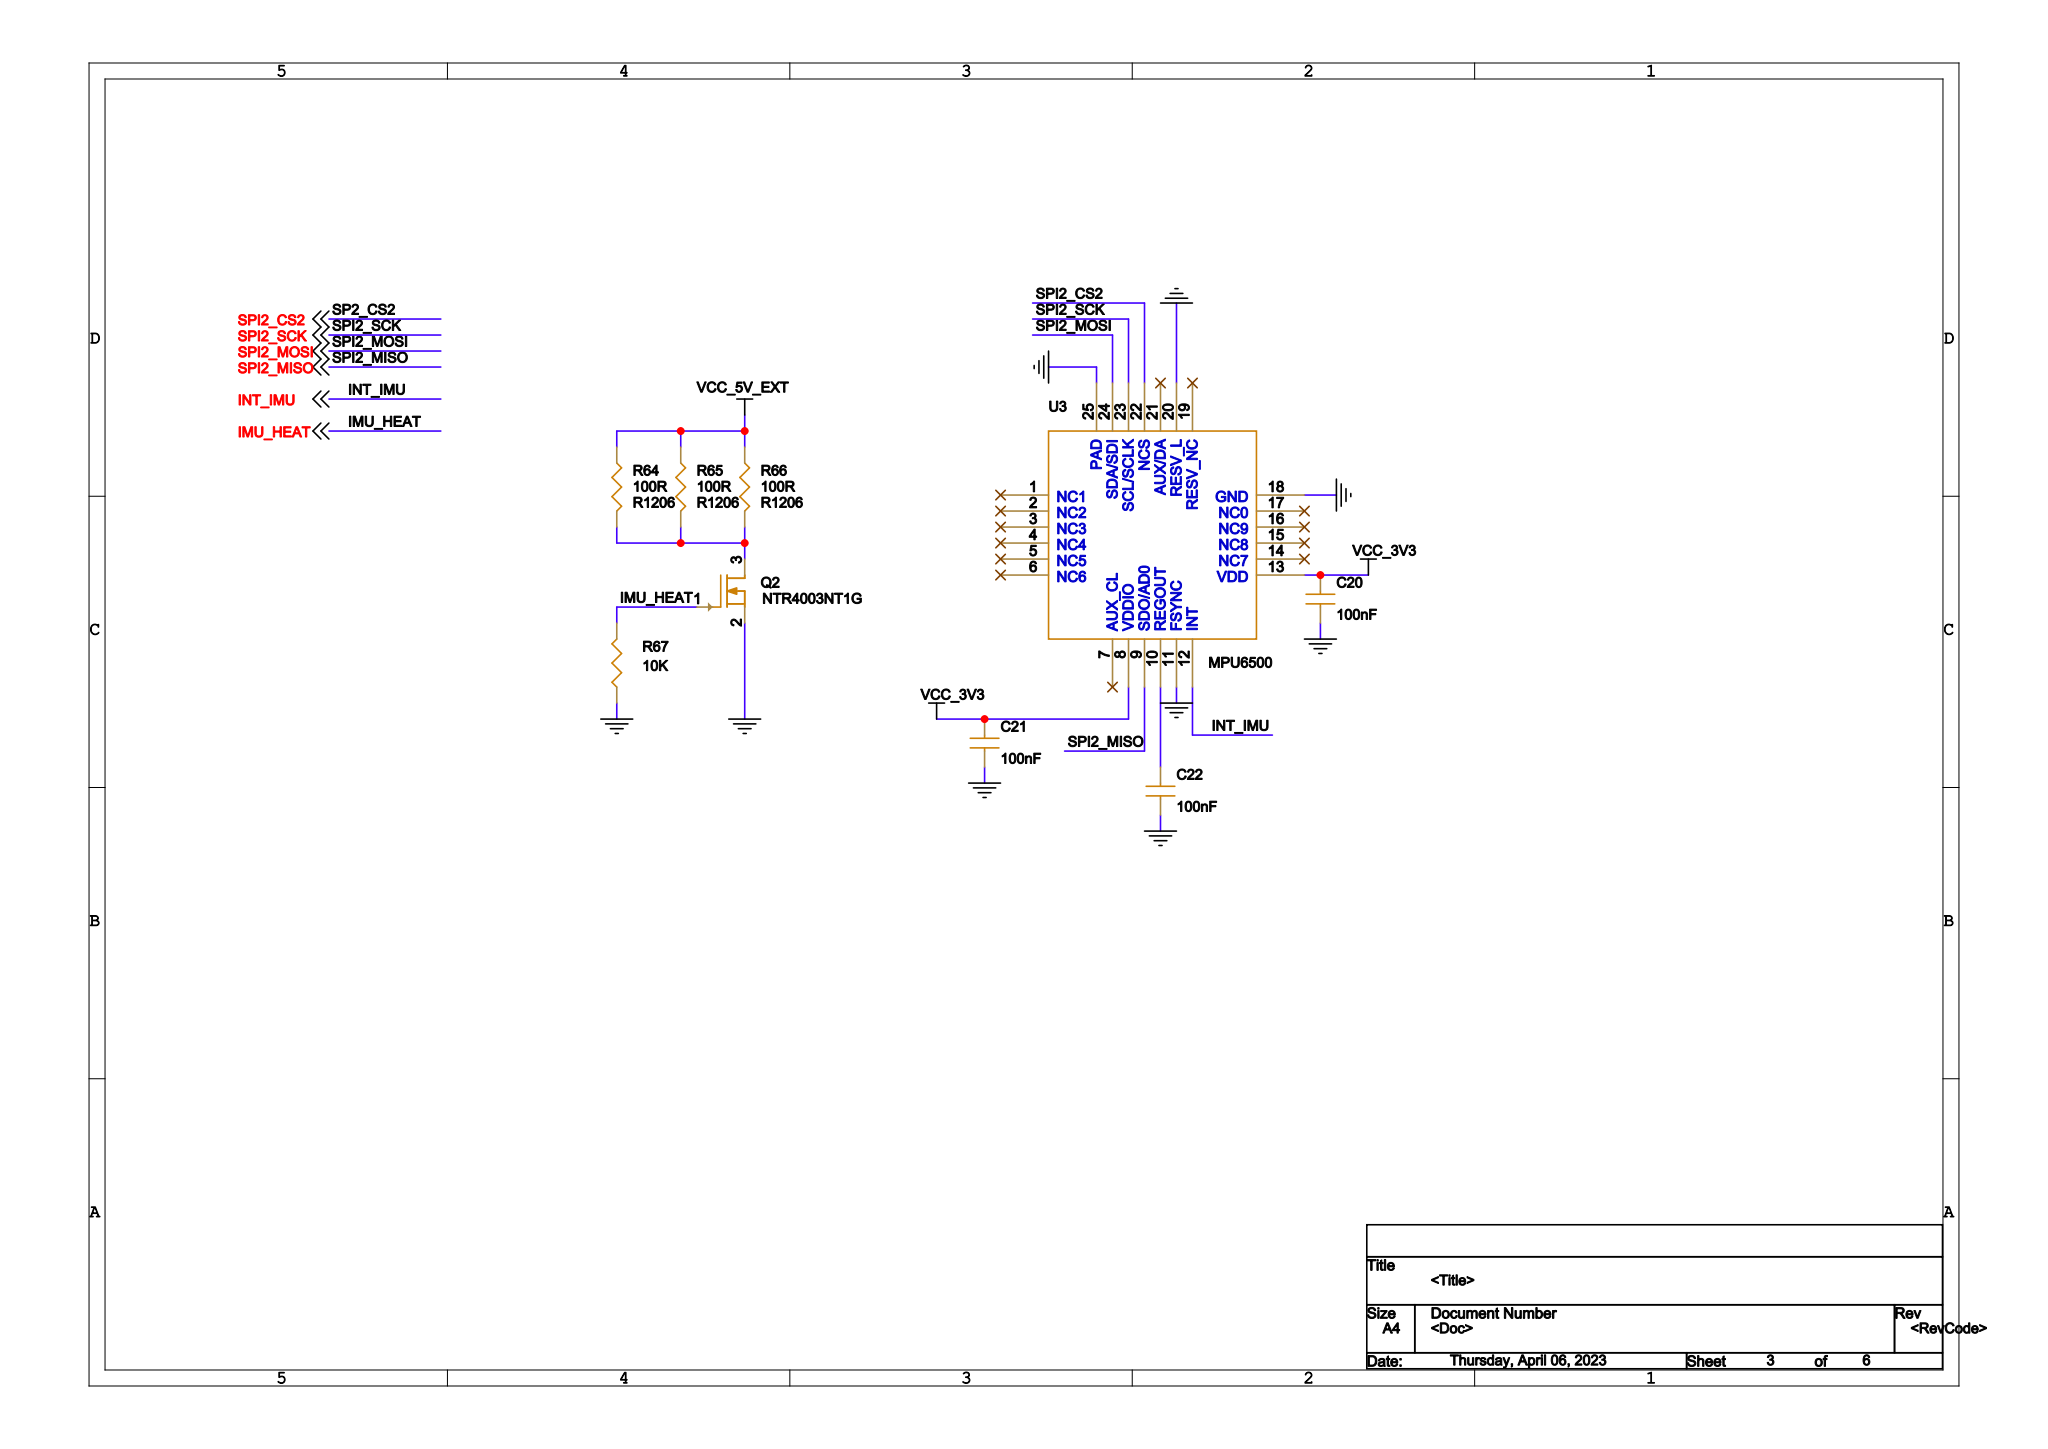Circuit board | Cadence Allegro | 278 parts | 154 nets | one sheet of the schematic
Parts on this sheet (reference | value | footprint):
C20 | 100nF | C0402
C21 | 100nF | C0402
C22 | 100nF | C0402
Q2 | NTR4003NT1G | SOT-23_0
R64 | 100R | R1206
R65 | 100R | R1206
R66 | 100R | R1206
R67 | 10K | R0402
U3 | MPU6500 | QFN
Nets of these parts (net: part-pin ...):
GND: C20-1 C21-1 C22-1 Q2-2 R67-1 U3-11 U3-18 U3-20 U3-25
VCC_3V3: C20-2 C21-2 U3-8 U3-13
N1031382: C22-2 U3-10
VCC_5V_EXT: R64-1 R65-1 R66-1
N1029307: Q2-3 R64-2 R65-2 R66-2
IMU_HEAT: Q2-1 R67-2
INT_IMU: U3-12
SPI2_MOSI: U3-24
SPI2_MISO: U3-9
SPI2_SCK: U3-23
SPI2_CS2: U3-22